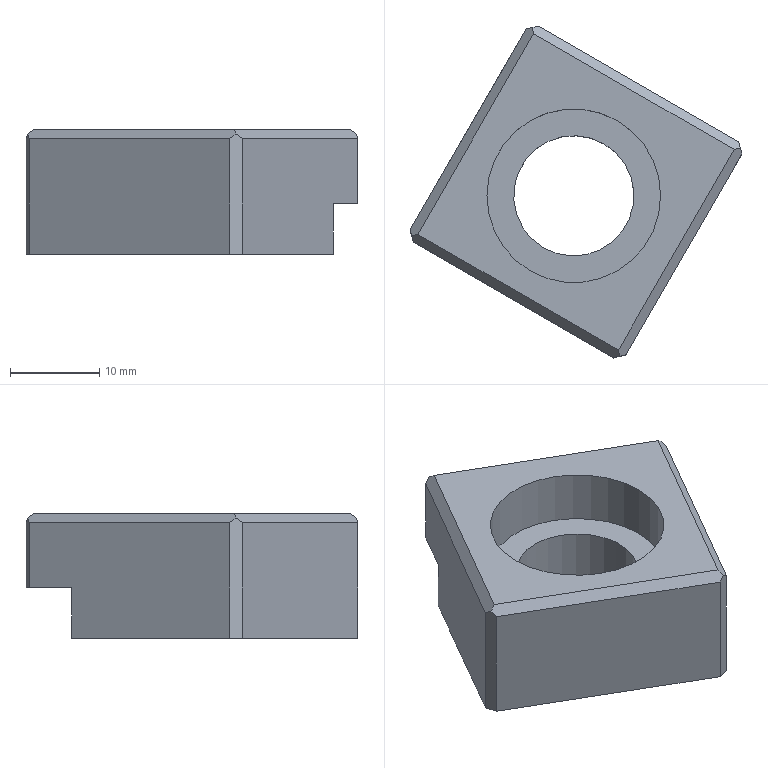Part | NX | features solid 2 | 1 solid | 19 faces | box 37.249 x 37.249 x 14 mm | volume 6926 mm3 | plane 17 | cylinder 2 | commonest cylinder face diameters 13.5 x1 19.5 x1
STEP:
#1=CARTESIAN_POINT('',(308.742,-378.141,232.7));
#2=VERTEX_POINT('',#1);
#3=CARTESIAN_POINT('',(308.742,-378.141,240.));
#4=VERTEX_POINT('',#3);
#5=CARTESIAN_POINT('',(308.742,-378.141,241.));
#6=DIRECTION('',(0.,0.,1.));
#7=VECTOR('',#6,1000.);
#8=LINE('',#5,#7);
#9=EDGE_CURVE('',#2,#4,#8,.T.);
#10=ORIENTED_EDGE('',*,*,#9,.T.);
#11=CARTESIAN_POINT('',(331.258,-391.141,240.));
#12=VERTEX_POINT('',#11);
#13=CARTESIAN_POINT('',(331.258,-391.141,240.));
#14=DIRECTION('',(0.866,-0.5,0.));
#15=VECTOR('',#14,1000.);
#16=LINE('',#13,#15);
#17=EDGE_CURVE('',#4,#12,#16,.T.);
#18=ORIENTED_EDGE('',*,*,#17,.T.);
#19=CARTESIAN_POINT('',(331.258,-391.141,232.7));
#20=VERTEX_POINT('',#19);
#21=CARTESIAN_POINT('',(331.258,-391.141,241.));
#22=DIRECTION('',(0.,0.,-1.));
#23=VECTOR('',#22,1000.);
#24=LINE('',#21,#23);
#25=EDGE_CURVE('',#12,#20,#24,.T.);
#26=ORIENTED_EDGE('',*,*,#25,.T.);
#27=CARTESIAN_POINT('',(307.876,-377.641,232.7));
#28=DIRECTION('',(0.866,-0.5,0.));
#29=VECTOR('',#28,1000.);
#30=LINE('',#27,#29);
#31=EDGE_CURVE('',#2,#20,#30,.T.);
#32=ORIENTED_EDGE('',*,*,#31,.F.);
#33=EDGE_LOOP('',(#10,#18,#26,#32));
#34=FACE_BOUND('',#33,.T.);
#35=CARTESIAN_POINT('',(307.876,-377.641,241.));
#36=DIRECTION('',(0.5,0.866,0.));
#37=DIRECTION('',(0.,0.,1.));
#38=AXIS2_PLACEMENT_3D('',#35,#36,#37);
#39=PLANE('',#38);
#40=ADVANCED_FACE('',(#34),#39,.T.);
#41=CARTESIAN_POINT('',(295.242,-401.524,241.));
#42=VERTEX_POINT('',#41);
#43=CARTESIAN_POINT('',(317.758,-414.524,241.));
#44=VERTEX_POINT('',#43);
#45=CARTESIAN_POINT('',(317.758,-414.524,241.));
#46=DIRECTION('',(0.866,-0.5,0.));
#47=VECTOR('',#46,1000.);
#48=LINE('',#45,#47);
#49=EDGE_CURVE('',#42,#44,#48,.T.);
#50=ORIENTED_EDGE('',*,*,#49,.T.);
#51=CARTESIAN_POINT('',(330.758,-392.007,241.));
#52=VERTEX_POINT('',#51);
#53=CARTESIAN_POINT('',(330.758,-392.007,241.));
#54=DIRECTION('',(0.5,0.866,0.));
#55=VECTOR('',#54,1000.);
#56=LINE('',#53,#55);
#57=EDGE_CURVE('',#44,#52,#56,.T.);
#58=ORIENTED_EDGE('',*,*,#57,.T.);
#59=CARTESIAN_POINT('',(308.242,-379.007,241.));
#60=VERTEX_POINT('',#59);
#61=CARTESIAN_POINT('',(308.242,-379.007,241.));
#62=DIRECTION('',(-0.866,0.5,0.));
#63=VECTOR('',#62,1000.);
#64=LINE('',#61,#63);
#65=EDGE_CURVE('',#52,#60,#64,.T.);
#66=ORIENTED_EDGE('',*,*,#65,.T.);
#67=CARTESIAN_POINT('',(295.242,-401.524,241.));
#68=DIRECTION('',(-0.5,-0.866,0.));
#69=VECTOR('',#68,1000.);
#70=LINE('',#67,#69);
#71=EDGE_CURVE('',#60,#42,#70,.T.);
#72=ORIENTED_EDGE('',*,*,#71,.T.);
#73=EDGE_LOOP('',(#50,#58,#66,#72));
#74=FACE_BOUND('',#73,.T.);
#75=CARTESIAN_POINT('',(307.875,-405.642,241.));
#76=VERTEX_POINT('',#75);
#77=CARTESIAN_POINT('',(312.75,-397.198,241.));
#78=DIRECTION('',(0.,0.,1.));
#79=DIRECTION('',(-0.5,-0.866,0.));
#80=AXIS2_PLACEMENT_3D('',#77,#78,#79);
#81=CIRCLE('',#80,9.75);
#82=EDGE_CURVE('',#76,#76,#81,.T.);
#83=ORIENTED_EDGE('',*,*,#82,.F.);
#84=EDGE_LOOP('',(#83));
#85=FACE_BOUND('',#84,.T.);
#86=CARTESIAN_POINT('',(293.876,-401.89,241.));
#87=DIRECTION('',(0.,0.,-1.));
#88=DIRECTION('',(0.5,0.866,0.));
#89=AXIS2_PLACEMENT_3D('',#86,#87,#88);
#90=PLANE('',#89);
#91=ADVANCED_FACE('',(#74,#85),#90,.F.);
#92=CARTESIAN_POINT('',(309.375,-403.044,227.));
#93=VERTEX_POINT('',#92);
#94=CARTESIAN_POINT('',(312.75,-397.198,227.));
#95=DIRECTION('',(0.,0.,1.));
#96=DIRECTION('',(-0.5,-0.866,0.));
#97=AXIS2_PLACEMENT_3D('',#94,#95,#96);
#98=CIRCLE('',#97,6.75);
#99=EDGE_CURVE('',#93,#93,#98,.T.);
#100=ORIENTED_EDGE('',*,*,#99,.F.);
#101=EDGE_LOOP('',(#100));
#102=FACE_BOUND('',#101,.T.);
#103=CARTESIAN_POINT('',(309.375,-403.044,235.));
#104=VERTEX_POINT('',#103);
#105=CARTESIAN_POINT('',(312.75,-397.198,235.));
#106=DIRECTION('',(0.,0.,1.));
#107=DIRECTION('',(-0.5,-0.866,0.));
#108=AXIS2_PLACEMENT_3D('',#105,#106,#107);
#109=CIRCLE('',#108,6.75);
#110=EDGE_CURVE('',#104,#104,#109,.T.);
#111=ORIENTED_EDGE('',*,*,#110,.T.);
#112=EDGE_LOOP('',(#111));
#113=FACE_BOUND('',#112,.T.);
#114=CARTESIAN_POINT('',(312.75,-397.198,247.));
#115=DIRECTION('',(0.,0.,-1.));
#116=DIRECTION('',(0.5,0.866,0.));
#117=AXIS2_PLACEMENT_3D('',#114,#115,#116);
#118=CYLINDRICAL_SURFACE('',#117,6.75);
#119=ADVANCED_FACE('',(#102,#113),#118,.F.);
#120=CARTESIAN_POINT('',(317.258,-415.39,227.));
#121=VERTEX_POINT('',#120);
#122=CARTESIAN_POINT('',(294.742,-402.39,227.));
#123=VERTEX_POINT('',#122);
#124=CARTESIAN_POINT('',(318.124,-415.89,227.));
#125=DIRECTION('',(-0.866,0.5,0.));
#126=VECTOR('',#125,1000.);
#127=LINE('',#124,#126);
#128=EDGE_CURVE('',#121,#123,#127,.T.);
#129=ORIENTED_EDGE('',*,*,#128,.T.);
#130=CARTESIAN_POINT('',(294.376,-401.024,227.));
#131=VERTEX_POINT('',#130);
#132=CARTESIAN_POINT('',(294.559,-401.707,227.));
#133=DIRECTION('',(0.2588,-0.9659,0.));
#134=VECTOR('',#133,1000.);
#135=LINE('',#132,#134);
#136=EDGE_CURVE('',#123,#131,#135,.F.);
#137=ORIENTED_EDGE('',*,*,#136,.T.);
#138=CARTESIAN_POINT('',(304.626,-383.27,227.));
#139=VERTEX_POINT('',#138);
#140=CARTESIAN_POINT('',(293.876,-401.89,227.));
#141=DIRECTION('',(0.5,0.866,0.));
#142=VECTOR('',#141,1000.);
#143=LINE('',#140,#142);
#144=EDGE_CURVE('',#131,#139,#143,.T.);
#145=ORIENTED_EDGE('',*,*,#144,.T.);
#146=CARTESIAN_POINT('',(328.874,-397.27,227.));
#147=VERTEX_POINT('',#146);
#148=CARTESIAN_POINT('',(328.874,-397.27,227.));
#149=DIRECTION('',(-0.866,0.5,0.));
#150=VECTOR('',#149,1000.);
#151=LINE('',#148,#150);
#152=EDGE_CURVE('',#147,#139,#151,.T.);
#153=ORIENTED_EDGE('',*,*,#152,.F.);
#154=CARTESIAN_POINT('',(318.624,-415.024,227.));
#155=VERTEX_POINT('',#154);
#156=CARTESIAN_POINT('',(332.124,-391.641,227.));
#157=DIRECTION('',(-0.5,-0.866,0.));
#158=VECTOR('',#157,1000.);
#159=LINE('',#156,#158);
#160=EDGE_CURVE('',#147,#155,#159,.T.);
#161=ORIENTED_EDGE('',*,*,#160,.T.);
#162=CARTESIAN_POINT('',(298.817,-420.331,227.));
#163=DIRECTION('',(0.9659,0.2588,0.));
#164=VECTOR('',#163,1000.);
#165=LINE('',#162,#164);
#166=EDGE_CURVE('',#155,#121,#165,.F.);
#167=ORIENTED_EDGE('',*,*,#166,.T.);
#168=EDGE_LOOP('',(#129,#137,#145,#153,#161,#167));
#169=FACE_BOUND('',#168,.T.);
#170=ORIENTED_EDGE('',*,*,#99,.T.);
#171=EDGE_LOOP('',(#170));
#172=FACE_BOUND('',#171,.T.);
#173=CARTESIAN_POINT('',(293.876,-401.89,227.));
#174=DIRECTION('',(0.,0.,-1.));
#175=DIRECTION('',(0.5,0.866,0.));
#176=AXIS2_PLACEMENT_3D('',#173,#174,#175);
#177=PLANE('',#176);
#178=ADVANCED_FACE('',(#169,#172),#177,.T.);
#179=CARTESIAN_POINT('',(317.258,-415.39,240.));
#180=VERTEX_POINT('',#179);
#181=CARTESIAN_POINT('',(317.258,-415.39,241.));
#182=DIRECTION('',(0.,0.,1.));
#183=VECTOR('',#182,1000.);
#184=LINE('',#181,#183);
#185=EDGE_CURVE('',#121,#180,#184,.T.);
#186=ORIENTED_EDGE('',*,*,#185,.T.);
#187=CARTESIAN_POINT('',(294.742,-402.39,240.));
#188=VERTEX_POINT('',#187);
#189=CARTESIAN_POINT('',(294.742,-402.39,240.));
#190=DIRECTION('',(-0.866,0.5,0.));
#191=VECTOR('',#190,1000.);
#192=LINE('',#189,#191);
#193=EDGE_CURVE('',#180,#188,#192,.T.);
#194=ORIENTED_EDGE('',*,*,#193,.T.);
#195=CARTESIAN_POINT('',(294.742,-402.39,241.));
#196=DIRECTION('',(0.,0.,-1.));
#197=VECTOR('',#196,1000.);
#198=LINE('',#195,#197);
#199=EDGE_CURVE('',#188,#123,#198,.T.);
#200=ORIENTED_EDGE('',*,*,#199,.T.);
#201=ORIENTED_EDGE('',*,*,#128,.F.);
#202=EDGE_LOOP('',(#186,#194,#200,#201));
#203=FACE_BOUND('',#202,.T.);
#204=CARTESIAN_POINT('',(318.124,-415.89,241.));
#205=DIRECTION('',(-0.5,-0.866,0.));
#206=DIRECTION('',(0.866,-0.5,0.));
#207=AXIS2_PLACEMENT_3D('',#204,#205,#206);
#208=PLANE('',#207);
#209=ADVANCED_FACE('',(#203),#208,.T.);
#210=CARTESIAN_POINT('',(294.376,-401.024,240.));
#211=VERTEX_POINT('',#210);
#212=CARTESIAN_POINT('',(294.376,-401.024,241.));
#213=DIRECTION('',(0.,0.,1.));
#214=VECTOR('',#213,1000.);
#215=LINE('',#212,#214);
#216=EDGE_CURVE('',#131,#211,#215,.T.);
#217=ORIENTED_EDGE('',*,*,#216,.T.);
#218=CARTESIAN_POINT('',(307.376,-378.507,240.));
#219=VERTEX_POINT('',#218);
#220=CARTESIAN_POINT('',(307.376,-378.507,240.));
#221=DIRECTION('',(0.5,0.866,0.));
#222=VECTOR('',#221,1000.);
#223=LINE('',#220,#222);
#224=EDGE_CURVE('',#211,#219,#223,.T.);
#225=ORIENTED_EDGE('',*,*,#224,.T.);
#226=CARTESIAN_POINT('',(307.376,-378.507,232.7));
#227=VERTEX_POINT('',#226);
#228=CARTESIAN_POINT('',(307.376,-378.507,241.));
#229=DIRECTION('',(0.,0.,-1.));
#230=VECTOR('',#229,1000.);
#231=LINE('',#228,#230);
#232=EDGE_CURVE('',#219,#227,#231,.T.);
#233=ORIENTED_EDGE('',*,*,#232,.T.);
#234=CARTESIAN_POINT('',(304.626,-383.27,232.7));
#235=VERTEX_POINT('',#234);
#236=CARTESIAN_POINT('',(304.626,-383.27,232.7));
#237=DIRECTION('',(0.5,0.866,0.));
#238=VECTOR('',#237,1000.);
#239=LINE('',#236,#238);
#240=EDGE_CURVE('',#235,#227,#239,.T.);
#241=ORIENTED_EDGE('',*,*,#240,.F.);
#242=CARTESIAN_POINT('',(304.626,-383.27,232.7));
#243=DIRECTION('',(0.,0.,-1.));
#244=VECTOR('',#243,1000.);
#245=LINE('',#242,#244);
#246=EDGE_CURVE('',#235,#139,#245,.T.);
#247=ORIENTED_EDGE('',*,*,#246,.T.);
#248=ORIENTED_EDGE('',*,*,#144,.F.);
#249=EDGE_LOOP('',(#217,#225,#233,#241,#247,#248));
#250=FACE_BOUND('',#249,.T.);
#251=CARTESIAN_POINT('',(293.876,-401.89,241.));
#252=DIRECTION('',(-0.866,0.5,0.));
#253=DIRECTION('',(-0.5,-0.866,0.));
#254=AXIS2_PLACEMENT_3D('',#251,#252,#253);
#255=PLANE('',#254);
#256=ADVANCED_FACE('',(#250),#255,.T.);
#257=CARTESIAN_POINT('',(331.624,-392.507,232.7));
#258=VERTEX_POINT('',#257);
#259=CARTESIAN_POINT('',(331.624,-392.507,240.));
#260=VERTEX_POINT('',#259);
#261=CARTESIAN_POINT('',(331.624,-392.507,241.));
#262=DIRECTION('',(0.,0.,1.));
#263=VECTOR('',#262,1000.);
#264=LINE('',#261,#263);
#265=EDGE_CURVE('',#258,#260,#264,.T.);
#266=ORIENTED_EDGE('',*,*,#265,.T.);
#267=CARTESIAN_POINT('',(318.624,-415.024,240.));
#268=VERTEX_POINT('',#267);
#269=CARTESIAN_POINT('',(318.624,-415.024,240.));
#270=DIRECTION('',(-0.5,-0.866,0.));
#271=VECTOR('',#270,1000.);
#272=LINE('',#269,#271);
#273=EDGE_CURVE('',#260,#268,#272,.T.);
#274=ORIENTED_EDGE('',*,*,#273,.T.);
#275=CARTESIAN_POINT('',(318.624,-415.024,241.));
#276=DIRECTION('',(0.,0.,-1.));
#277=VECTOR('',#276,1000.);
#278=LINE('',#275,#277);
#279=EDGE_CURVE('',#268,#155,#278,.T.);
#280=ORIENTED_EDGE('',*,*,#279,.T.);
#281=ORIENTED_EDGE('',*,*,#160,.F.);
#282=CARTESIAN_POINT('',(328.874,-397.27,232.7));
#283=VERTEX_POINT('',#282);
#284=CARTESIAN_POINT('',(328.874,-397.27,232.7));
#285=DIRECTION('',(0.,0.,-1.));
#286=VECTOR('',#285,1000.);
#287=LINE('',#284,#286);
#288=EDGE_CURVE('',#283,#147,#287,.T.);
#289=ORIENTED_EDGE('',*,*,#288,.F.);
#290=CARTESIAN_POINT('',(328.874,-397.27,232.7));
#291=DIRECTION('',(0.5,0.866,0.));
#292=VECTOR('',#291,1000.);
#293=LINE('',#290,#292);
#294=EDGE_CURVE('',#283,#258,#293,.T.);
#295=ORIENTED_EDGE('',*,*,#294,.T.);
#296=EDGE_LOOP('',(#266,#274,#280,#281,#289,#295));
#297=FACE_BOUND('',#296,.T.);
#298=CARTESIAN_POINT('',(332.124,-391.641,241.));
#299=DIRECTION('',(0.866,-0.5,0.));
#300=DIRECTION('',(0.,0.,1.));
#301=AXIS2_PLACEMENT_3D('',#298,#299,#300);
#302=PLANE('',#301);
#303=ADVANCED_FACE('',(#297),#302,.T.);
#304=ORIENTED_EDGE('',*,*,#82,.T.);
#305=EDGE_LOOP('',(#304));
#306=FACE_BOUND('',#305,.T.);
#307=CARTESIAN_POINT('',(307.875,-405.642,235.));
#308=VERTEX_POINT('',#307);
#309=CARTESIAN_POINT('',(312.75,-397.198,235.));
#310=DIRECTION('',(0.,0.,1.));
#311=DIRECTION('',(-0.5,-0.866,0.));
#312=AXIS2_PLACEMENT_3D('',#309,#310,#311);
#313=CIRCLE('',#312,9.75);
#314=EDGE_CURVE('',#308,#308,#313,.T.);
#315=ORIENTED_EDGE('',*,*,#314,.F.);
#316=EDGE_LOOP('',(#315));
#317=FACE_BOUND('',#316,.T.);
#318=CARTESIAN_POINT('',(312.75,-397.198,241.));
#319=DIRECTION('',(0.,0.,-1.));
#320=DIRECTION('',(0.5,0.866,0.));
#321=AXIS2_PLACEMENT_3D('',#318,#319,#320);
#322=CYLINDRICAL_SURFACE('',#321,9.75);
#323=ADVANCED_FACE('',(#306,#317),#322,.F.);
#324=ORIENTED_EDGE('',*,*,#110,.F.);
#325=EDGE_LOOP('',(#324));
#326=FACE_BOUND('',#325,.T.);
#327=ORIENTED_EDGE('',*,*,#314,.T.);
#328=EDGE_LOOP('',(#327));
#329=FACE_BOUND('',#328,.T.);
#330=CARTESIAN_POINT('',(312.75,-397.198,235.));
#331=DIRECTION('',(0.,0.,1.));
#332=DIRECTION('',(-0.5,-0.866,0.));
#333=AXIS2_PLACEMENT_3D('',#330,#331,#332);
#334=PLANE('',#333);
#335=ADVANCED_FACE('',(#326,#329),#334,.T.);
#336=ORIENTED_EDGE('',*,*,#152,.T.);
#337=ORIENTED_EDGE('',*,*,#246,.F.);
#338=CARTESIAN_POINT('',(328.874,-397.27,232.7));
#339=DIRECTION('',(-0.866,0.5,0.));
#340=VECTOR('',#339,1000.);
#341=LINE('',#338,#340);
#342=EDGE_CURVE('',#283,#235,#341,.T.);
#343=ORIENTED_EDGE('',*,*,#342,.F.);
#344=ORIENTED_EDGE('',*,*,#288,.T.);
#345=EDGE_LOOP('',(#336,#337,#343,#344));
#346=FACE_BOUND('',#345,.T.);
#347=CARTESIAN_POINT('',(328.874,-397.27,232.7));
#348=DIRECTION('',(-0.5,-0.866,0.));
#349=DIRECTION('',(0.866,-0.5,0.));
#350=AXIS2_PLACEMENT_3D('',#347,#348,#349);
#351=PLANE('',#350);
#352=ADVANCED_FACE('',(#346),#351,.F.);
#353=ORIENTED_EDGE('',*,*,#240,.T.);
#354=CARTESIAN_POINT('',(327.183,-373.2,232.7));
#355=DIRECTION('',(-0.9659,-0.2588,0.));
#356=VECTOR('',#355,1000.);
#357=LINE('',#354,#356);
#358=EDGE_CURVE('',#227,#2,#357,.F.);
#359=ORIENTED_EDGE('',*,*,#358,.T.);
#360=ORIENTED_EDGE('',*,*,#31,.T.);
#361=CARTESIAN_POINT('',(331.441,-391.824,232.7));
#362=DIRECTION('',(-0.2588,0.9659,0.));
#363=VECTOR('',#362,1000.);
#364=LINE('',#361,#363);
#365=EDGE_CURVE('',#20,#258,#364,.F.);
#366=ORIENTED_EDGE('',*,*,#365,.T.);
#367=ORIENTED_EDGE('',*,*,#294,.F.);
#368=ORIENTED_EDGE('',*,*,#342,.T.);
#369=EDGE_LOOP('',(#353,#359,#360,#366,#367,#368));
#370=FACE_BOUND('',#369,.T.);
#371=CARTESIAN_POINT('',(332.124,-391.641,232.7));
#372=DIRECTION('',(0.,0.,-1.));
#373=DIRECTION('',(0.5,0.866,0.));
#374=AXIS2_PLACEMENT_3D('',#371,#372,#373);
#375=PLANE('',#374);
#376=ADVANCED_FACE('',(#370),#375,.T.);
#377=CARTESIAN_POINT('',(294.559,-401.707,240.5));
#378=VERTEX_POINT('',#377);
#379=CARTESIAN_POINT('',(294.62,-401.934,240.333));
#380=DIRECTION('',(0.2113,-0.7887,-0.5774));
#381=VECTOR('',#380,1000.);
#382=LINE('',#379,#381);
#383=EDGE_CURVE('',#188,#378,#382,.F.);
#384=ORIENTED_EDGE('',*,*,#383,.T.);
#385=CARTESIAN_POINT('',(294.742,-402.39,241.));
#386=DIRECTION('',(0.2113,-0.7887,0.5774));
#387=VECTOR('',#386,1000.);
#388=LINE('',#385,#387);
#389=EDGE_CURVE('',#378,#211,#388,.F.);
#390=ORIENTED_EDGE('',*,*,#389,.T.);
#391=ORIENTED_EDGE('',*,*,#216,.F.);
#392=ORIENTED_EDGE('',*,*,#136,.F.);
#393=ORIENTED_EDGE('',*,*,#199,.F.);
#394=EDGE_LOOP('',(#384,#390,#391,#392,#393));
#395=FACE_BOUND('',#394,.T.);
#396=CARTESIAN_POINT('',(294.742,-402.39,241.));
#397=DIRECTION('',(0.9659,0.2588,0.));
#398=DIRECTION('',(-0.2588,0.9659,0.));
#399=AXIS2_PLACEMENT_3D('',#396,#397,#398);
#400=PLANE('',#399);
#401=ADVANCED_FACE('',(#395),#400,.F.);
#402=ORIENTED_EDGE('',*,*,#232,.F.);
#403=CARTESIAN_POINT('',(308.059,-378.324,240.5));
#404=VERTEX_POINT('',#403);
#405=CARTESIAN_POINT('',(307.831,-378.385,240.333));
#406=DIRECTION('',(-0.7887,-0.2113,-0.5774));
#407=VECTOR('',#406,1000.);
#408=LINE('',#405,#407);
#409=EDGE_CURVE('',#219,#404,#408,.F.);
#410=ORIENTED_EDGE('',*,*,#409,.T.);
#411=CARTESIAN_POINT('',(307.376,-378.507,241.));
#412=DIRECTION('',(-0.7887,-0.2113,0.5774));
#413=VECTOR('',#412,1000.);
#414=LINE('',#411,#413);
#415=EDGE_CURVE('',#404,#4,#414,.F.);
#416=ORIENTED_EDGE('',*,*,#415,.T.);
#417=ORIENTED_EDGE('',*,*,#9,.F.);
#418=ORIENTED_EDGE('',*,*,#358,.F.);
#419=EDGE_LOOP('',(#402,#410,#416,#417,#418));
#420=FACE_BOUND('',#419,.T.);
#421=CARTESIAN_POINT('',(307.376,-378.507,241.));
#422=DIRECTION('',(0.2588,-0.9659,0.));
#423=DIRECTION('',(0.9659,0.2588,0.));
#424=AXIS2_PLACEMENT_3D('',#421,#422,#423);
#425=PLANE('',#424);
#426=ADVANCED_FACE('',(#420),#425,.F.);
#427=ORIENTED_EDGE('',*,*,#279,.F.);
#428=CARTESIAN_POINT('',(317.941,-415.207,240.5));
#429=VERTEX_POINT('',#428);
#430=CARTESIAN_POINT('',(318.169,-415.146,240.333));
#431=DIRECTION('',(0.7887,0.2113,-0.5774));
#432=VECTOR('',#431,1000.);
#433=LINE('',#430,#432);
#434=EDGE_CURVE('',#268,#429,#433,.F.);
#435=ORIENTED_EDGE('',*,*,#434,.T.);
#436=CARTESIAN_POINT('',(318.624,-415.024,241.));
#437=DIRECTION('',(0.7887,0.2113,0.5774));
#438=VECTOR('',#437,1000.);
#439=LINE('',#436,#438);
#440=EDGE_CURVE('',#429,#180,#439,.F.);
#441=ORIENTED_EDGE('',*,*,#440,.T.);
#442=ORIENTED_EDGE('',*,*,#185,.F.);
#443=ORIENTED_EDGE('',*,*,#166,.F.);
#444=EDGE_LOOP('',(#427,#435,#441,#442,#443));
#445=FACE_BOUND('',#444,.T.);
#446=CARTESIAN_POINT('',(318.624,-415.024,241.));
#447=DIRECTION('',(-0.2588,0.9659,0.));
#448=DIRECTION('',(-0.9659,-0.2588,0.));
#449=AXIS2_PLACEMENT_3D('',#446,#447,#448);
#450=PLANE('',#449);
#451=ADVANCED_FACE('',(#445),#450,.F.);
#452=CARTESIAN_POINT('',(331.441,-391.824,240.5));
#453=VERTEX_POINT('',#452);
#454=CARTESIAN_POINT('',(331.38,-391.596,240.333));
#455=DIRECTION('',(-0.2113,0.7887,-0.5774));
#456=VECTOR('',#455,1000.);
#457=LINE('',#454,#456);
#458=EDGE_CURVE('',#12,#453,#457,.F.);
#459=ORIENTED_EDGE('',*,*,#458,.T.);
#460=CARTESIAN_POINT('',(331.258,-391.141,241.));
#461=DIRECTION('',(-0.2113,0.7887,0.5774));
#462=VECTOR('',#461,1000.);
#463=LINE('',#460,#462);
#464=EDGE_CURVE('',#453,#260,#463,.F.);
#465=ORIENTED_EDGE('',*,*,#464,.T.);
#466=ORIENTED_EDGE('',*,*,#265,.F.);
#467=ORIENTED_EDGE('',*,*,#365,.F.);
#468=ORIENTED_EDGE('',*,*,#25,.F.);
#469=EDGE_LOOP('',(#459,#465,#466,#467,#468));
#470=FACE_BOUND('',#469,.T.);
#471=CARTESIAN_POINT('',(331.258,-391.141,241.));
#472=DIRECTION('',(-0.9659,-0.2588,0.));
#473=DIRECTION('',(0.2588,-0.9659,0.));
#474=AXIS2_PLACEMENT_3D('',#471,#472,#473);
#475=PLANE('',#474);
#476=ADVANCED_FACE('',(#470),#475,.F.);
#477=ORIENTED_EDGE('',*,*,#440,.F.);
#478=CARTESIAN_POINT('',(318.124,-415.89,240.));
#479=DIRECTION('',(-0.2113,0.7887,0.5774));
#480=VECTOR('',#479,1000.);
#481=LINE('',#478,#480);
#482=EDGE_CURVE('',#429,#44,#481,.T.);
#483=ORIENTED_EDGE('',*,*,#482,.T.);
#484=ORIENTED_EDGE('',*,*,#49,.F.);
#485=CARTESIAN_POINT('',(306.625,-398.473,249.333));
#486=DIRECTION('',(-0.7887,-0.2113,-0.5774));
#487=VECTOR('',#486,1000.);
#488=LINE('',#485,#487);
#489=EDGE_CURVE('',#42,#378,#488,.T.);
#490=ORIENTED_EDGE('',*,*,#489,.T.);
#491=ORIENTED_EDGE('',*,*,#383,.F.);
#492=ORIENTED_EDGE('',*,*,#193,.F.);
#493=EDGE_LOOP('',(#477,#483,#484,#490,#491,#492));
#494=FACE_BOUND('',#493,.T.);
#495=CARTESIAN_POINT('',(318.124,-415.89,240.));
#496=DIRECTION('',(-0.3536,-0.6124,0.7071));
#497=DIRECTION('',(-0.3536,-0.6124,-0.7071));
#498=AXIS2_PLACEMENT_3D('',#495,#496,#497);
#499=PLANE('',#498);
#500=ADVANCED_FACE('',(#494),#499,.T.);
#501=ORIENTED_EDGE('',*,*,#65,.F.);
#502=CARTESIAN_POINT('',(319.375,-395.057,249.333));
#503=DIRECTION('',(0.7887,0.2113,-0.5774));
#504=VECTOR('',#503,1000.);
#505=LINE('',#502,#504);
#506=EDGE_CURVE('',#52,#453,#505,.T.);
#507=ORIENTED_EDGE('',*,*,#506,.T.);
#508=ORIENTED_EDGE('',*,*,#458,.F.);
#509=ORIENTED_EDGE('',*,*,#17,.F.);
#510=ORIENTED_EDGE('',*,*,#415,.F.);
#511=CARTESIAN_POINT('',(307.876,-377.641,240.));
#512=DIRECTION('',(0.2113,-0.7887,0.5774));
#513=VECTOR('',#512,1000.);
#514=LINE('',#511,#513);
#515=EDGE_CURVE('',#404,#60,#514,.T.);
#516=ORIENTED_EDGE('',*,*,#515,.T.);
#517=EDGE_LOOP('',(#501,#507,#508,#509,#510,#516));
#518=FACE_BOUND('',#517,.T.);
#519=CARTESIAN_POINT('',(307.876,-377.641,240.));
#520=DIRECTION('',(0.3536,0.6124,0.7071));
#521=DIRECTION('',(-0.3536,-0.6124,0.7071));
#522=AXIS2_PLACEMENT_3D('',#519,#520,#521);
#523=PLANE('',#522);
#524=ADVANCED_FACE('',(#518),#523,.T.);
#525=ORIENTED_EDGE('',*,*,#506,.F.);
#526=ORIENTED_EDGE('',*,*,#57,.F.);
#527=ORIENTED_EDGE('',*,*,#482,.F.);
#528=ORIENTED_EDGE('',*,*,#434,.F.);
#529=ORIENTED_EDGE('',*,*,#273,.F.);
#530=ORIENTED_EDGE('',*,*,#464,.F.);
#531=EDGE_LOOP('',(#525,#526,#527,#528,#529,#530));
#532=FACE_BOUND('',#531,.T.);
#533=CARTESIAN_POINT('',(332.124,-391.641,240.));
#534=DIRECTION('',(0.6124,-0.3536,0.7071));
#535=DIRECTION('',(-0.6124,0.3536,0.7071));
#536=AXIS2_PLACEMENT_3D('',#533,#534,#535);
#537=PLANE('',#536);
#538=ADVANCED_FACE('',(#532),#537,.T.);
#539=ORIENTED_EDGE('',*,*,#489,.F.);
#540=ORIENTED_EDGE('',*,*,#71,.F.);
#541=ORIENTED_EDGE('',*,*,#515,.F.);
#542=ORIENTED_EDGE('',*,*,#409,.F.);
#543=ORIENTED_EDGE('',*,*,#224,.F.);
#544=ORIENTED_EDGE('',*,*,#389,.F.);
#545=EDGE_LOOP('',(#539,#540,#541,#542,#543,#544));
#546=FACE_BOUND('',#545,.T.);
#547=CARTESIAN_POINT('',(293.876,-401.89,240.));
#548=DIRECTION('',(-0.6124,0.3536,0.7071));
#549=DIRECTION('',(-0.6124,0.3536,-0.7071));
#550=AXIS2_PLACEMENT_3D('',#547,#548,#549);
#551=PLANE('',#550);
#552=ADVANCED_FACE('',(#546),#551,.T.);
#553=CLOSED_SHELL('',(#40,#91,#119,#178,#209,#256,#303,#323,#335,#352,#376,#401,#426,#451,#476,#500,#524,#538,#552));
#554=MANIFOLD_SOLID_BREP('',#553);
#555=(LENGTH_UNIT()NAMED_UNIT(*)SI_UNIT(.MILLI.,.METRE.));
#556=UNCERTAINTY_MEASURE_WITH_UNIT(LENGTH_MEASURE(0.00001),#555,'','');
#557=(NAMED_UNIT(*)PLANE_ANGLE_UNIT()SI_UNIT($,.RADIAN.));
#558=(NAMED_UNIT(*)SI_UNIT($,.STERADIAN.)SOLID_ANGLE_UNIT());
#559=(GEOMETRIC_REPRESENTATION_CONTEXT(3)GLOBAL_UNCERTAINTY_ASSIGNED_CONTEXT((#556))GLOBAL_UNIT_ASSIGNED_CONTEXT((#555,#557,#558))REPRESENTATION_CONTEXT('',''));
#560=ADVANCED_BREP_SHAPE_REPRESENTATION('',(#554),#559);